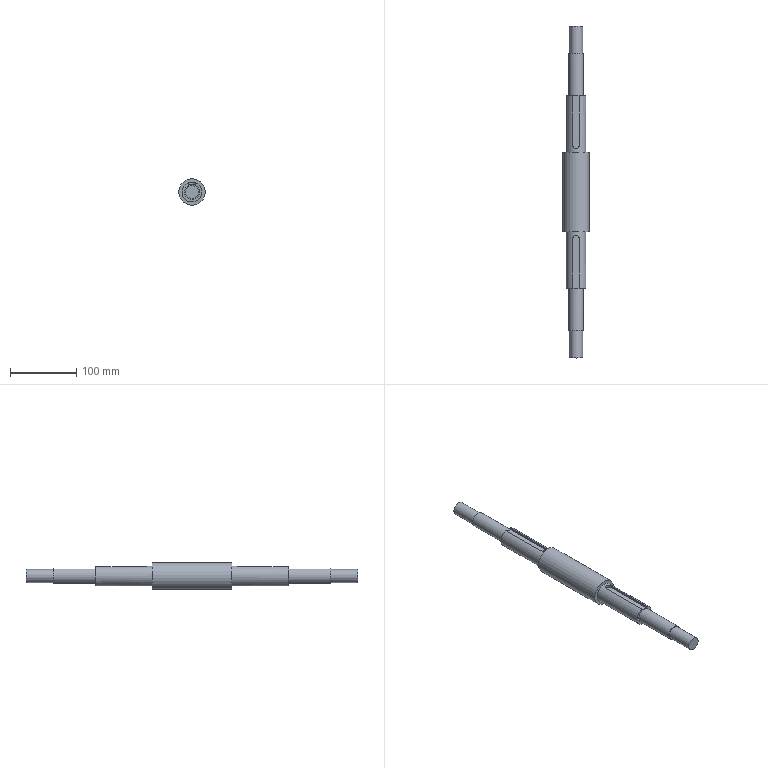Part | STEP file | SN10_001_006_EIXO | 1 solid | 25 faces | box 40 x 500.1 x 40 mm | volume 341783 mm3 | plane 16 | cylinder 9 | commonest cylinder face diameters 10 x2 20 x2 22.5 x2 30 x2 40 x1